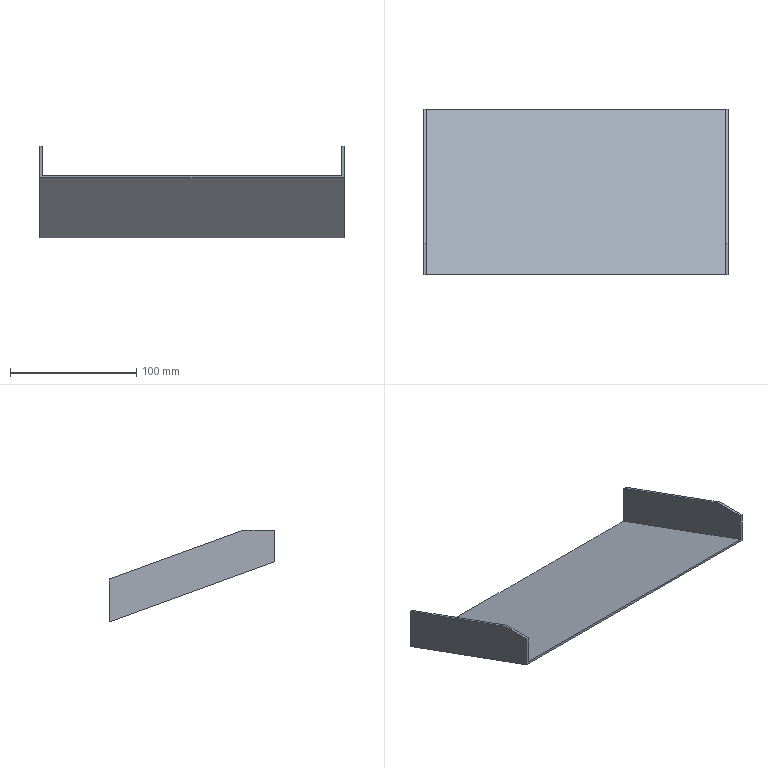Part | NX | features HB 2 | 1 solid | 12 faces | box 241 x 131 x 72.795 mm | volume 83484 mm3 | plane 12
STEP:
#1=CARTESIAN_POINT('',(493.54,-256.,-213.));
#2=VERTEX_POINT('',#1);
#3=CARTESIAN_POINT('',(493.54,-231.44,-213.));
#4=VERTEX_POINT('',#3);
#5=CARTESIAN_POINT('',(493.54,-20.77,-213.));
#6=DIRECTION('',(0.,1.,0.));
#7=VECTOR('',#6,1000.);
#8=LINE('',#5,#7);
#9=EDGE_CURVE('',#2,#4,#8,.T.);
#10=ORIENTED_EDGE('',*,*,#9,.F.);
#11=CARTESIAN_POINT('',(493.54,-256.,-238.115));
#12=VERTEX_POINT('',#11);
#13=CARTESIAN_POINT('',(493.54,-256.,-321.603));
#14=DIRECTION('',(0.,0.,1.));
#15=VECTOR('',#14,1000.);
#16=LINE('',#13,#15);
#17=EDGE_CURVE('',#12,#2,#16,.T.);
#18=ORIENTED_EDGE('',*,*,#17,.F.);
#19=CARTESIAN_POINT('',(493.54,-125.,-285.795));
#20=VERTEX_POINT('',#19);
#21=CARTESIAN_POINT('',(493.54,-21.454,-323.482));
#22=DIRECTION('',(0.,0.9397,-0.342));
#23=VECTOR('',#22,1000.);
#24=LINE('',#21,#23);
#25=EDGE_CURVE('',#12,#20,#24,.T.);
#26=ORIENTED_EDGE('',*,*,#25,.T.);
#27=CARTESIAN_POINT('',(493.54,-125.,-251.741));
#28=VERTEX_POINT('',#27);
#29=CARTESIAN_POINT('',(493.54,-125.,-321.603));
#30=DIRECTION('',(0.,0.,1.));
#31=VECTOR('',#30,1000.);
#32=LINE('',#29,#31);
#33=EDGE_CURVE('',#20,#28,#32,.T.);
#34=ORIENTED_EDGE('',*,*,#33,.T.);
#35=CARTESIAN_POINT('',(493.54,-10.51,-293.412));
#36=DIRECTION('',(0.,-0.9397,0.342));
#37=VECTOR('',#36,1000.);
#38=LINE('',#35,#37);
#39=EDGE_CURVE('',#28,#4,#38,.T.);
#40=ORIENTED_EDGE('',*,*,#39,.T.);
#41=EDGE_LOOP('',(#10,#18,#26,#34,#40));
#42=FACE_BOUND('',#41,.T.);
#43=CARTESIAN_POINT('',(493.54,-20.77,-321.603));
#44=DIRECTION('',(-1.,0.,0.));
#45=DIRECTION('',(0.,0.08716,-0.9962));
#46=AXIS2_PLACEMENT_3D('',#43,#44,#45);
#47=PLANE('',#46);
#48=ADVANCED_FACE('',(#42),#47,.F.);
#49=CARTESIAN_POINT('',(252.54,-231.44,-213.));
#50=VERTEX_POINT('',#49);
#51=CARTESIAN_POINT('',(252.54,-256.,-213.));
#52=VERTEX_POINT('',#51);
#53=CARTESIAN_POINT('',(252.54,-20.77,-213.));
#54=DIRECTION('',(0.,-1.,0.));
#55=VECTOR('',#54,1000.);
#56=LINE('',#53,#55);
#57=EDGE_CURVE('',#50,#52,#56,.T.);
#58=ORIENTED_EDGE('',*,*,#57,.F.);
#59=CARTESIAN_POINT('',(252.54,-125.,-251.741));
#60=VERTEX_POINT('',#59);
#61=CARTESIAN_POINT('',(252.54,-10.51,-293.412));
#62=DIRECTION('',(0.,-0.9397,0.342));
#63=VECTOR('',#62,1000.);
#64=LINE('',#61,#63);
#65=EDGE_CURVE('',#60,#50,#64,.T.);
#66=ORIENTED_EDGE('',*,*,#65,.F.);
#67=CARTESIAN_POINT('',(252.54,-125.,-285.795));
#68=VERTEX_POINT('',#67);
#69=CARTESIAN_POINT('',(252.54,-125.,-321.603));
#70=DIRECTION('',(0.,0.,-1.));
#71=VECTOR('',#70,1000.);
#72=LINE('',#69,#71);
#73=EDGE_CURVE('',#60,#68,#72,.T.);
#74=ORIENTED_EDGE('',*,*,#73,.T.);
#75=CARTESIAN_POINT('',(252.54,-256.,-238.115));
#76=VERTEX_POINT('',#75);
#77=CARTESIAN_POINT('',(252.54,-21.454,-323.482));
#78=DIRECTION('',(0.,-0.9397,0.342));
#79=VECTOR('',#78,1000.);
#80=LINE('',#77,#79);
#81=EDGE_CURVE('',#68,#76,#80,.T.);
#82=ORIENTED_EDGE('',*,*,#81,.T.);
#83=CARTESIAN_POINT('',(252.54,-256.,-321.603));
#84=DIRECTION('',(0.,0.,-1.));
#85=VECTOR('',#84,1000.);
#86=LINE('',#83,#85);
#87=EDGE_CURVE('',#52,#76,#86,.T.);
#88=ORIENTED_EDGE('',*,*,#87,.F.);
#89=EDGE_LOOP('',(#58,#66,#74,#82,#88));
#90=FACE_BOUND('',#89,.T.);
#91=CARTESIAN_POINT('',(252.54,-20.77,-321.603));
#92=DIRECTION('',(1.,0.,0.));
#93=DIRECTION('',(0.,-0.08716,0.9962));
#94=AXIS2_PLACEMENT_3D('',#91,#92,#93);
#95=PLANE('',#94);
#96=ADVANCED_FACE('',(#90),#95,.F.);
#97=CARTESIAN_POINT('',(254.54,-125.,-251.741));
#98=VERTEX_POINT('',#97);
#99=CARTESIAN_POINT('',(254.54,-231.44,-213.));
#100=VERTEX_POINT('',#99);
#101=CARTESIAN_POINT('',(254.54,-10.51,-293.412));
#102=DIRECTION('',(0.,-0.9397,0.342));
#103=VECTOR('',#102,1000.);
#104=LINE('',#101,#103);
#105=EDGE_CURVE('',#98,#100,#104,.T.);
#106=ORIENTED_EDGE('',*,*,#105,.T.);
#107=CARTESIAN_POINT('',(254.54,-256.,-213.));
#108=VERTEX_POINT('',#107);
#109=CARTESIAN_POINT('',(254.54,-20.77,-213.));
#110=DIRECTION('',(0.,-1.,0.));
#111=VECTOR('',#110,1000.);
#112=LINE('',#109,#111);
#113=EDGE_CURVE('',#100,#108,#112,.T.);
#114=ORIENTED_EDGE('',*,*,#113,.T.);
#115=CARTESIAN_POINT('',(254.54,-256.,-235.986));
#116=VERTEX_POINT('',#115);
#117=CARTESIAN_POINT('',(254.54,-256.,-321.603));
#118=DIRECTION('',(0.,0.,-1.));
#119=VECTOR('',#118,1000.);
#120=LINE('',#117,#119);
#121=EDGE_CURVE('',#108,#116,#120,.T.);
#122=ORIENTED_EDGE('',*,*,#121,.T.);
#123=CARTESIAN_POINT('',(254.54,-125.,-283.666));
#124=VERTEX_POINT('',#123);
#125=CARTESIAN_POINT('',(254.54,-20.77,-321.603));
#126=DIRECTION('',(0.,0.9397,-0.342));
#127=VECTOR('',#126,1000.);
#128=LINE('',#125,#127);
#129=EDGE_CURVE('',#116,#124,#128,.T.);
#130=ORIENTED_EDGE('',*,*,#129,.T.);
#131=CARTESIAN_POINT('',(254.54,-125.,-321.603));
#132=DIRECTION('',(0.,0.,-1.));
#133=VECTOR('',#132,1000.);
#134=LINE('',#131,#133);
#135=EDGE_CURVE('',#98,#124,#134,.T.);
#136=ORIENTED_EDGE('',*,*,#135,.F.);
#137=EDGE_LOOP('',(#106,#114,#122,#130,#136));
#138=FACE_BOUND('',#137,.T.);
#139=CARTESIAN_POINT('',(254.54,-20.77,-321.603));
#140=DIRECTION('',(1.,0.,0.));
#141=DIRECTION('',(0.,-0.08716,0.9962));
#142=AXIS2_PLACEMENT_3D('',#139,#140,#141);
#143=PLANE('',#142);
#144=ADVANCED_FACE('',(#138),#143,.T.);
#145=CARTESIAN_POINT('',(491.54,-256.,-235.986));
#146=VERTEX_POINT('',#145);
#147=CARTESIAN_POINT('',(491.54,-256.,-213.));
#148=VERTEX_POINT('',#147);
#149=CARTESIAN_POINT('',(491.54,-256.,-321.603));
#150=DIRECTION('',(0.,0.,1.));
#151=VECTOR('',#150,1000.);
#152=LINE('',#149,#151);
#153=EDGE_CURVE('',#146,#148,#152,.T.);
#154=ORIENTED_EDGE('',*,*,#153,.T.);
#155=CARTESIAN_POINT('',(491.54,-231.44,-213.));
#156=VERTEX_POINT('',#155);
#157=CARTESIAN_POINT('',(491.54,-20.77,-213.));
#158=DIRECTION('',(0.,1.,0.));
#159=VECTOR('',#158,1000.);
#160=LINE('',#157,#159);
#161=EDGE_CURVE('',#148,#156,#160,.T.);
#162=ORIENTED_EDGE('',*,*,#161,.T.);
#163=CARTESIAN_POINT('',(491.54,-125.,-251.741));
#164=VERTEX_POINT('',#163);
#165=CARTESIAN_POINT('',(491.54,-10.51,-293.412));
#166=DIRECTION('',(0.,-0.9397,0.342));
#167=VECTOR('',#166,1000.);
#168=LINE('',#165,#167);
#169=EDGE_CURVE('',#164,#156,#168,.T.);
#170=ORIENTED_EDGE('',*,*,#169,.F.);
#171=CARTESIAN_POINT('',(491.54,-125.,-283.666));
#172=VERTEX_POINT('',#171);
#173=CARTESIAN_POINT('',(491.54,-125.,-321.603));
#174=DIRECTION('',(0.,0.,1.));
#175=VECTOR('',#174,1000.);
#176=LINE('',#173,#175);
#177=EDGE_CURVE('',#172,#164,#176,.T.);
#178=ORIENTED_EDGE('',*,*,#177,.F.);
#179=CARTESIAN_POINT('',(491.54,-20.77,-321.603));
#180=DIRECTION('',(0.,-0.9397,0.342));
#181=VECTOR('',#180,1000.);
#182=LINE('',#179,#181);
#183=EDGE_CURVE('',#172,#146,#182,.T.);
#184=ORIENTED_EDGE('',*,*,#183,.T.);
#185=EDGE_LOOP('',(#154,#162,#170,#178,#184));
#186=FACE_BOUND('',#185,.T.);
#187=CARTESIAN_POINT('',(491.54,-20.77,-321.603));
#188=DIRECTION('',(-1.,0.,0.));
#189=DIRECTION('',(0.,-0.08716,0.9962));
#190=AXIS2_PLACEMENT_3D('',#187,#188,#189);
#191=PLANE('',#190);
#192=ADVANCED_FACE('',(#186),#191,.T.);
#193=CARTESIAN_POINT('',(254.54,-231.44,-213.));
#194=DIRECTION('',(-1.,0.,0.));
#195=VECTOR('',#194,1000.);
#196=LINE('',#193,#195);
#197=EDGE_CURVE('',#100,#50,#196,.T.);
#198=ORIENTED_EDGE('',*,*,#197,.F.);
#199=ORIENTED_EDGE('',*,*,#105,.F.);
#200=CARTESIAN_POINT('',(254.54,-125.,-251.741));
#201=DIRECTION('',(-1.,0.,0.));
#202=VECTOR('',#201,1000.);
#203=LINE('',#200,#202);
#204=EDGE_CURVE('',#98,#60,#203,.T.);
#205=ORIENTED_EDGE('',*,*,#204,.T.);
#206=ORIENTED_EDGE('',*,*,#65,.T.);
#207=EDGE_LOOP('',(#198,#199,#205,#206));
#208=FACE_BOUND('',#207,.T.);
#209=CARTESIAN_POINT('',(254.54,-10.51,-293.412));
#210=DIRECTION('',(0.,-0.342,-0.9397));
#211=DIRECTION('',(0.,0.9397,-0.342));
#212=AXIS2_PLACEMENT_3D('',#209,#210,#211);
#213=PLANE('',#212);
#214=ADVANCED_FACE('',(#208),#213,.F.);
#215=CARTESIAN_POINT('',(601.54,-231.44,-213.));
#216=DIRECTION('',(-1.,0.,0.));
#217=VECTOR('',#216,1000.);
#218=LINE('',#215,#217);
#219=EDGE_CURVE('',#4,#156,#218,.T.);
#220=ORIENTED_EDGE('',*,*,#219,.F.);
#221=ORIENTED_EDGE('',*,*,#39,.F.);
#222=CARTESIAN_POINT('',(601.54,-125.,-251.741));
#223=DIRECTION('',(-1.,0.,0.));
#224=VECTOR('',#223,1000.);
#225=LINE('',#222,#224);
#226=EDGE_CURVE('',#28,#164,#225,.T.);
#227=ORIENTED_EDGE('',*,*,#226,.T.);
#228=ORIENTED_EDGE('',*,*,#169,.T.);
#229=EDGE_LOOP('',(#220,#221,#227,#228));
#230=FACE_BOUND('',#229,.T.);
#231=CARTESIAN_POINT('',(601.54,-10.51,-293.412));
#232=DIRECTION('',(0.,-0.342,-0.9397));
#233=DIRECTION('',(0.,0.9397,-0.342));
#234=AXIS2_PLACEMENT_3D('',#231,#232,#233);
#235=PLANE('',#234);
#236=ADVANCED_FACE('',(#230),#235,.F.);
#237=ORIENTED_EDGE('',*,*,#17,.T.);
#238=CARTESIAN_POINT('',(116.,-256.,-213.));
#239=DIRECTION('',(-1.,0.,0.));
#240=VECTOR('',#239,1000.);
#241=LINE('',#238,#240);
#242=EDGE_CURVE('',#2,#148,#241,.T.);
#243=ORIENTED_EDGE('',*,*,#242,.T.);
#244=ORIENTED_EDGE('',*,*,#153,.F.);
#245=CARTESIAN_POINT('',(496.54,-256.,-235.986));
#246=DIRECTION('',(1.,0.,0.));
#247=VECTOR('',#246,1000.);
#248=LINE('',#245,#247);
#249=EDGE_CURVE('',#116,#146,#248,.T.);
#250=ORIENTED_EDGE('',*,*,#249,.F.);
#251=ORIENTED_EDGE('',*,*,#121,.F.);
#252=CARTESIAN_POINT('',(106.,-256.,-213.));
#253=DIRECTION('',(-1.,0.,0.));
#254=VECTOR('',#253,1000.);
#255=LINE('',#252,#254);
#256=EDGE_CURVE('',#108,#52,#255,.T.);
#257=ORIENTED_EDGE('',*,*,#256,.T.);
#258=ORIENTED_EDGE('',*,*,#87,.T.);
#259=CARTESIAN_POINT('',(496.54,-256.,-238.115));
#260=DIRECTION('',(1.,0.,0.));
#261=VECTOR('',#260,1000.);
#262=LINE('',#259,#261);
#263=EDGE_CURVE('',#76,#12,#262,.T.);
#264=ORIENTED_EDGE('',*,*,#263,.T.);
#265=EDGE_LOOP('',(#237,#243,#244,#250,#251,#257,#258,#264));
#266=FACE_BOUND('',#265,.T.);
#267=CARTESIAN_POINT('',(116.,-256.,55.));
#268=DIRECTION('',(0.,-1.,0.));
#269=DIRECTION('',(0.,0.,1.));
#270=AXIS2_PLACEMENT_3D('',#267,#268,#269);
#271=PLANE('',#270);
#272=ADVANCED_FACE('',(#266),#271,.T.);
#273=ORIENTED_EDGE('',*,*,#129,.F.);
#274=ORIENTED_EDGE('',*,*,#249,.T.);
#275=ORIENTED_EDGE('',*,*,#183,.F.);
#276=CARTESIAN_POINT('',(496.54,-125.,-283.666));
#277=DIRECTION('',(1.,0.,0.));
#278=VECTOR('',#277,1000.);
#279=LINE('',#276,#278);
#280=EDGE_CURVE('',#124,#172,#279,.T.);
#281=ORIENTED_EDGE('',*,*,#280,.F.);
#282=EDGE_LOOP('',(#273,#274,#275,#281));
#283=FACE_BOUND('',#282,.T.);
#284=CARTESIAN_POINT('',(496.54,-20.77,-321.603));
#285=DIRECTION('',(0.,0.342,0.9397));
#286=DIRECTION('',(-1.,0.,0.));
#287=AXIS2_PLACEMENT_3D('',#284,#285,#286);
#288=PLANE('',#287);
#289=ADVANCED_FACE('',(#283),#288,.T.);
#290=ORIENTED_EDGE('',*,*,#263,.F.);
#291=ORIENTED_EDGE('',*,*,#81,.F.);
#292=CARTESIAN_POINT('',(496.54,-125.,-285.795));
#293=DIRECTION('',(1.,0.,0.));
#294=VECTOR('',#293,1000.);
#295=LINE('',#292,#294);
#296=EDGE_CURVE('',#68,#20,#295,.T.);
#297=ORIENTED_EDGE('',*,*,#296,.T.);
#298=ORIENTED_EDGE('',*,*,#25,.F.);
#299=EDGE_LOOP('',(#290,#291,#297,#298));
#300=FACE_BOUND('',#299,.T.);
#301=CARTESIAN_POINT('',(496.54,-21.454,-323.482));
#302=DIRECTION('',(0.,0.342,0.9397));
#303=DIRECTION('',(-1.,0.,0.));
#304=AXIS2_PLACEMENT_3D('',#301,#302,#303);
#305=PLANE('',#304);
#306=ADVANCED_FACE('',(#300),#305,.F.);
#307=ORIENTED_EDGE('',*,*,#280,.T.);
#308=ORIENTED_EDGE('',*,*,#177,.T.);
#309=ORIENTED_EDGE('',*,*,#226,.F.);
#310=ORIENTED_EDGE('',*,*,#33,.F.);
#311=ORIENTED_EDGE('',*,*,#296,.F.);
#312=ORIENTED_EDGE('',*,*,#73,.F.);
#313=ORIENTED_EDGE('',*,*,#204,.F.);
#314=ORIENTED_EDGE('',*,*,#135,.T.);
#315=EDGE_LOOP('',(#307,#308,#309,#310,#311,#312,#313,#314));
#316=FACE_BOUND('',#315,.T.);
#317=CARTESIAN_POINT('',(733.,-125.,-2175.5));
#318=DIRECTION('',(0.,-1.,0.));
#319=DIRECTION('',(0.,0.,-1.));
#320=AXIS2_PLACEMENT_3D('',#317,#318,#319);
#321=PLANE('',#320);
#322=ADVANCED_FACE('',(#316),#321,.F.);
#323=ORIENTED_EDGE('',*,*,#113,.F.);
#324=ORIENTED_EDGE('',*,*,#197,.T.);
#325=ORIENTED_EDGE('',*,*,#57,.T.);
#326=ORIENTED_EDGE('',*,*,#256,.F.);
#327=EDGE_LOOP('',(#323,#324,#325,#326));
#328=FACE_BOUND('',#327,.T.);
#329=CARTESIAN_POINT('',(1935.,0.,-213.));
#330=DIRECTION('',(0.,0.,1.));
#331=DIRECTION('',(-1.,0.,0.));
#332=AXIS2_PLACEMENT_3D('',#329,#330,#331);
#333=PLANE('',#332);
#334=ADVANCED_FACE('',(#328),#333,.T.);
#335=ORIENTED_EDGE('',*,*,#9,.T.);
#336=ORIENTED_EDGE('',*,*,#219,.T.);
#337=ORIENTED_EDGE('',*,*,#161,.F.);
#338=ORIENTED_EDGE('',*,*,#242,.F.);
#339=EDGE_LOOP('',(#335,#336,#337,#338));
#340=FACE_BOUND('',#339,.T.);
#341=CARTESIAN_POINT('',(1945.,0.,-213.));
#342=DIRECTION('',(0.,0.,1.));
#343=DIRECTION('',(-1.,0.,0.));
#344=AXIS2_PLACEMENT_3D('',#341,#342,#343);
#345=PLANE('',#344);
#346=ADVANCED_FACE('',(#340),#345,.T.);
#347=CLOSED_SHELL('',(#48,#96,#144,#192,#214,#236,#272,#289,#306,#322,#334,#346));
#348=MANIFOLD_SOLID_BREP('',#347);
#349=(LENGTH_UNIT()NAMED_UNIT(*)SI_UNIT(.MILLI.,.METRE.));
#350=UNCERTAINTY_MEASURE_WITH_UNIT(LENGTH_MEASURE(0.00001),#349,'','');
#351=(NAMED_UNIT(*)PLANE_ANGLE_UNIT()SI_UNIT($,.RADIAN.));
#352=(NAMED_UNIT(*)SI_UNIT($,.STERADIAN.)SOLID_ANGLE_UNIT());
#353=(GEOMETRIC_REPRESENTATION_CONTEXT(3)GLOBAL_UNCERTAINTY_ASSIGNED_CONTEXT((#350))GLOBAL_UNIT_ASSIGNED_CONTEXT((#349,#351,#352))REPRESENTATION_CONTEXT('',''));
#354=ADVANCED_BREP_SHAPE_REPRESENTATION('',(#348),#353);